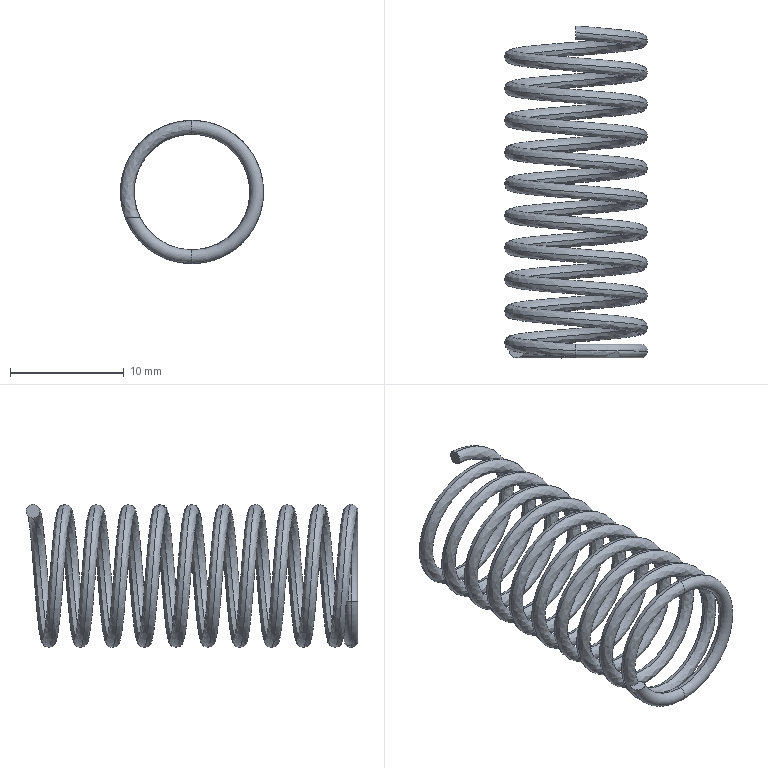Part | SolidWorks | features Helix 1, ICE 1, Revolution 1, Sweep 1 | 1 solid | 8 faces | box 12.6 x 29.2 x 12.6 mm | volume 432.63 mm3 | torus 4 | spline 2 | plane 2